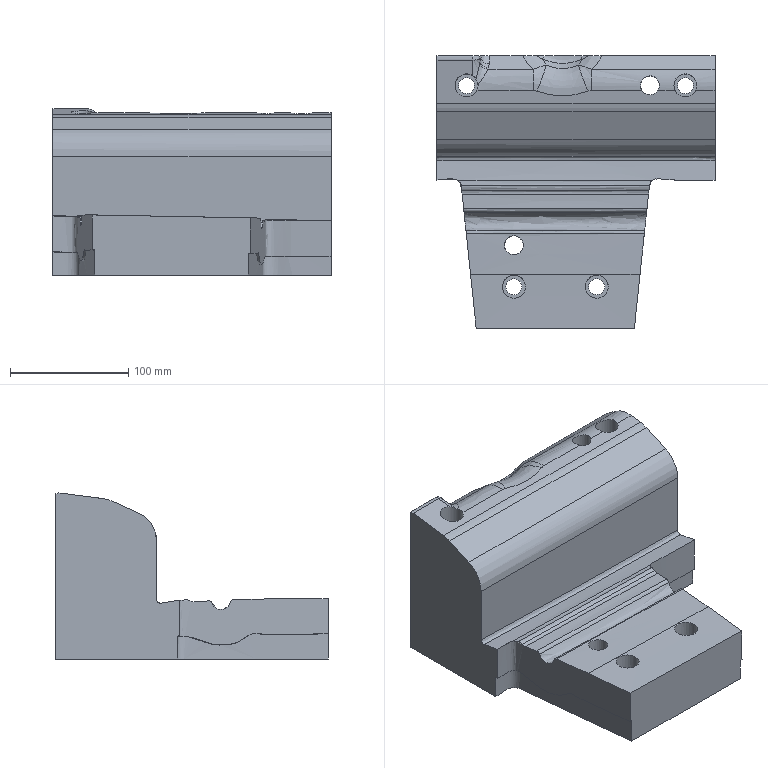Part | NX | features solid 2 | 1 solid | 64 faces | box 235.003 x 230 x 140.328 mm | volume 3527982 mm3 | spline 45 | cylinder 10 | plane 9 | commonest cylinder face diameters 13.5 x4 19.5 x4 16 x2